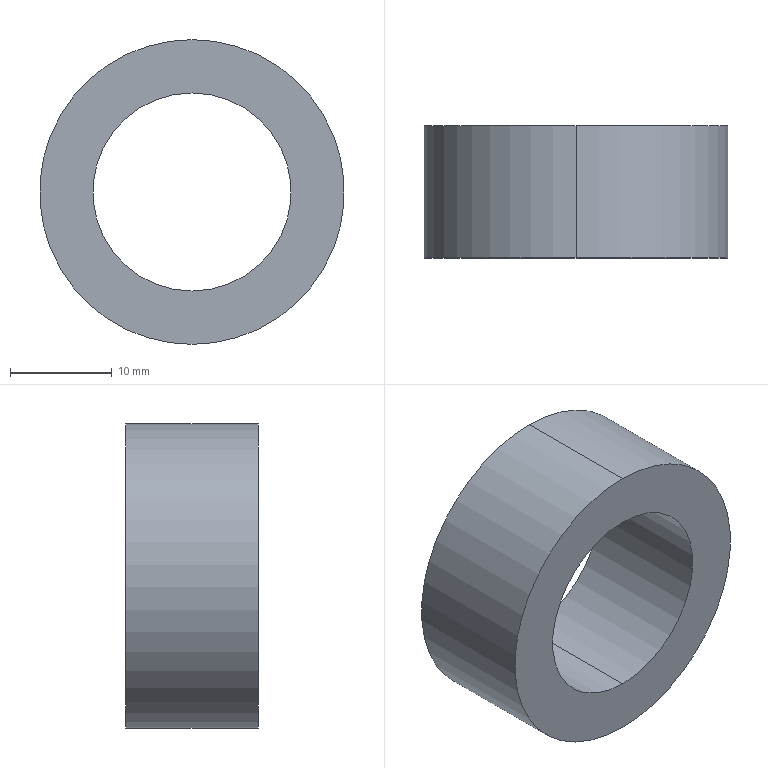Part | STEP file | Polyurethane washer | 1 solid | 6 faces | box 30 x 13 x 30 mm | volume 5307 mm3 | cylinder 4 | plane 2 | commonest cylinder face diameters 19.5 x2 30 x2
STEP:
#1=CARTESIAN_POINT('',(0.,0.,0.));
#2=DIRECTION('',(0.,0.,1.));
#3=DIRECTION('',(1.,0.,0.));
#4=AXIS2_PLACEMENT_3D('',#1,#2,#3);
#5=CARTESIAN_POINT('',(0.,13.,-9.75));
#6=VERTEX_POINT('',#5);
#7=CARTESIAN_POINT('',(0.,0.,-9.75));
#8=VERTEX_POINT('',#7);
#9=CARTESIAN_POINT('',(0.,13.,-9.75));
#10=DIRECTION('',(0.,-1.,0.));
#11=VECTOR('',#10,1.);
#12=LINE('',#9,#11);
#13=CARTESIAN_POINT('',(0.,13.,0.));
#14=DIRECTION('',(0.,-1.,0.));
#15=DIRECTION('',(0.,0.,-1.));
#16=AXIS2_PLACEMENT_3D('',#13,#14,#15);
#17=CYLINDRICAL_SURFACE('',#16,9.75);
#18=CARTESIAN_POINT('',(6.283,0.));
#19=DIRECTION('',(0.,1.));
#20=VECTOR('',#19,1.);
#21=LINE('',#18,#20);
#22=(GEOMETRIC_REPRESENTATION_CONTEXT(2)PARAMETRIC_REPRESENTATION_CONTEXT()REPRESENTATION_CONTEXT('',''));
#23=DEFINITIONAL_REPRESENTATION('',(#21),#22);
#24=PCURVE('',#17,#23);
#25=CARTESIAN_POINT('',(0.,13.,0.));
#26=DIRECTION('',(0.,-1.,0.));
#27=DIRECTION('',(0.,0.,-1.));
#28=AXIS2_PLACEMENT_3D('',#25,#26,#27);
#29=CYLINDRICAL_SURFACE('',#28,9.75);
#30=CARTESIAN_POINT('',(0.,0.));
#31=DIRECTION('',(0.,1.));
#32=VECTOR('',#31,1.);
#33=LINE('',#30,#32);
#34=(GEOMETRIC_REPRESENTATION_CONTEXT(2)PARAMETRIC_REPRESENTATION_CONTEXT()REPRESENTATION_CONTEXT('',''));
#35=DEFINITIONAL_REPRESENTATION('',(#33),#34);
#36=PCURVE('',#29,#35);
#37=SURFACE_CURVE('',#12,(#24,#36),.PCURVE_S1.);
#38=EDGE_CURVE('',#6,#8,#37,.T.);
#39=ORIENTED_EDGE('',*,*,#38,.T.);
#40=CARTESIAN_POINT('',(0.,0.,9.75));
#41=VERTEX_POINT('',#40);
#42=CARTESIAN_POINT('',(0.,0.,0.));
#43=DIRECTION('',(0.,1.,0.));
#44=DIRECTION('',(0.,0.,1.));
#45=AXIS2_PLACEMENT_3D('',#42,#43,#44);
#46=CIRCLE('',#45,9.75);
#47=CARTESIAN_POINT('',(9.425,13.));
#48=DIRECTION('',(-1.,0.));
#49=VECTOR('',#48,1.);
#50=LINE('',#47,#49);
#51=(GEOMETRIC_REPRESENTATION_CONTEXT(2)PARAMETRIC_REPRESENTATION_CONTEXT()REPRESENTATION_CONTEXT('',''));
#52=DEFINITIONAL_REPRESENTATION('',(#50),#51);
#53=PCURVE('',#17,#52);
#54=CARTESIAN_POINT('',(0.,0.,0.));
#55=DIRECTION('',(0.,1.,0.));
#56=DIRECTION('',(0.,0.,1.));
#57=AXIS2_PLACEMENT_3D('',#54,#55,#56);
#58=PLANE('',#57);
#59=CARTESIAN_POINT('',(0.,0.));
#60=DIRECTION('',(1.,0.));
#61=AXIS2_PLACEMENT_2D('',#59,#60);
#62=CIRCLE('',#61,9.75);
#63=(GEOMETRIC_REPRESENTATION_CONTEXT(2)PARAMETRIC_REPRESENTATION_CONTEXT()REPRESENTATION_CONTEXT('',''));
#64=DEFINITIONAL_REPRESENTATION('',(#62),#63);
#65=PCURVE('',#58,#64);
#66=SURFACE_CURVE('',#46,(#53,#65),.PCURVE_S1.);
#67=EDGE_CURVE('',#8,#41,#66,.T.);
#68=ORIENTED_EDGE('',*,*,#67,.T.);
#69=CARTESIAN_POINT('',(0.,13.,9.75));
#70=VERTEX_POINT('',#69);
#71=CARTESIAN_POINT('',(0.,13.,9.75));
#72=DIRECTION('',(0.,-1.,0.));
#73=VECTOR('',#72,1.);
#74=LINE('',#71,#73);
#75=CARTESIAN_POINT('',(3.142,0.));
#76=DIRECTION('',(0.,1.));
#77=VECTOR('',#76,1.);
#78=LINE('',#75,#77);
#79=(GEOMETRIC_REPRESENTATION_CONTEXT(2)PARAMETRIC_REPRESENTATION_CONTEXT()REPRESENTATION_CONTEXT('',''));
#80=DEFINITIONAL_REPRESENTATION('',(#78),#79);
#81=PCURVE('',#17,#80);
#82=CARTESIAN_POINT('',(3.142,0.));
#83=DIRECTION('',(0.,1.));
#84=VECTOR('',#83,1.);
#85=LINE('',#82,#84);
#86=(GEOMETRIC_REPRESENTATION_CONTEXT(2)PARAMETRIC_REPRESENTATION_CONTEXT()REPRESENTATION_CONTEXT('',''));
#87=DEFINITIONAL_REPRESENTATION('',(#85),#86);
#88=PCURVE('',#29,#87);
#89=SURFACE_CURVE('',#74,(#81,#88),.PCURVE_S1.);
#90=EDGE_CURVE('',#70,#41,#89,.T.);
#91=ORIENTED_EDGE('',*,*,#90,.F.);
#92=CARTESIAN_POINT('',(0.,13.,0.));
#93=DIRECTION('',(0.,1.,0.));
#94=DIRECTION('',(0.,0.,1.));
#95=AXIS2_PLACEMENT_3D('',#92,#93,#94);
#96=CIRCLE('',#95,9.75);
#97=CARTESIAN_POINT('',(9.425,0.));
#98=DIRECTION('',(-1.,0.));
#99=VECTOR('',#98,1.);
#100=LINE('',#97,#99);
#101=(GEOMETRIC_REPRESENTATION_CONTEXT(2)PARAMETRIC_REPRESENTATION_CONTEXT()REPRESENTATION_CONTEXT('',''));
#102=DEFINITIONAL_REPRESENTATION('',(#100),#101);
#103=PCURVE('',#17,#102);
#104=CARTESIAN_POINT('',(0.,13.,0.));
#105=DIRECTION('',(0.,1.,0.));
#106=DIRECTION('',(0.,0.,1.));
#107=AXIS2_PLACEMENT_3D('',#104,#105,#106);
#108=PLANE('',#107);
#109=CARTESIAN_POINT('',(0.,0.));
#110=DIRECTION('',(1.,0.));
#111=AXIS2_PLACEMENT_2D('',#109,#110);
#112=CIRCLE('',#111,9.75);
#113=(GEOMETRIC_REPRESENTATION_CONTEXT(2)PARAMETRIC_REPRESENTATION_CONTEXT()REPRESENTATION_CONTEXT('',''));
#114=DEFINITIONAL_REPRESENTATION('',(#112),#113);
#115=PCURVE('',#108,#114);
#116=SURFACE_CURVE('',#96,(#103,#115),.PCURVE_S1.);
#117=EDGE_CURVE('',#6,#70,#116,.T.);
#118=ORIENTED_EDGE('',*,*,#117,.F.);
#119=EDGE_LOOP('',(#39,#68,#91,#118));
#120=FACE_BOUND('',#119,.F.);
#121=ADVANCED_FACE('',(#120),#17,.F.);
#122=CARTESIAN_POINT('',(0.,13.,15.));
#123=VERTEX_POINT('',#122);
#124=CARTESIAN_POINT('',(0.,13.,-15.));
#125=VERTEX_POINT('',#124);
#126=CARTESIAN_POINT('',(0.,13.,0.));
#127=DIRECTION('',(0.,1.,0.));
#128=DIRECTION('',(0.,0.,1.));
#129=AXIS2_PLACEMENT_3D('',#126,#127,#128);
#130=CIRCLE('',#129,15.);
#131=CARTESIAN_POINT('',(0.,13.,0.));
#132=DIRECTION('',(0.,-1.,0.));
#133=DIRECTION('',(0.,0.,-1.));
#134=AXIS2_PLACEMENT_3D('',#131,#132,#133);
#135=CYLINDRICAL_SURFACE('',#134,15.);
#136=CARTESIAN_POINT('',(3.142,0.));
#137=DIRECTION('',(-1.,0.));
#138=VECTOR('',#137,1.);
#139=LINE('',#136,#138);
#140=(GEOMETRIC_REPRESENTATION_CONTEXT(2)PARAMETRIC_REPRESENTATION_CONTEXT()REPRESENTATION_CONTEXT('',''));
#141=DEFINITIONAL_REPRESENTATION('',(#139),#140);
#142=PCURVE('',#135,#141);
#143=CARTESIAN_POINT('',(0.,0.));
#144=DIRECTION('',(1.,0.));
#145=AXIS2_PLACEMENT_2D('',#143,#144);
#146=CIRCLE('',#145,15.);
#147=(GEOMETRIC_REPRESENTATION_CONTEXT(2)PARAMETRIC_REPRESENTATION_CONTEXT()REPRESENTATION_CONTEXT('',''));
#148=DEFINITIONAL_REPRESENTATION('',(#146),#147);
#149=PCURVE('',#108,#148);
#150=SURFACE_CURVE('',#130,(#142,#149),.PCURVE_S1.);
#151=EDGE_CURVE('',#123,#125,#150,.T.);
#152=ORIENTED_EDGE('',*,*,#151,.F.);
#153=CARTESIAN_POINT('',(0.,0.,15.));
#154=VERTEX_POINT('',#153);
#155=CARTESIAN_POINT('',(0.,13.,15.));
#156=DIRECTION('',(0.,-1.,0.));
#157=VECTOR('',#156,1.);
#158=LINE('',#155,#157);
#159=CARTESIAN_POINT('',(3.142,0.));
#160=DIRECTION('',(0.,1.));
#161=VECTOR('',#160,1.);
#162=LINE('',#159,#161);
#163=(GEOMETRIC_REPRESENTATION_CONTEXT(2)PARAMETRIC_REPRESENTATION_CONTEXT()REPRESENTATION_CONTEXT('',''));
#164=DEFINITIONAL_REPRESENTATION('',(#162),#163);
#165=PCURVE('',#135,#164);
#166=CARTESIAN_POINT('',(0.,13.,0.));
#167=DIRECTION('',(0.,-1.,0.));
#168=DIRECTION('',(0.,0.,-1.));
#169=AXIS2_PLACEMENT_3D('',#166,#167,#168);
#170=CYLINDRICAL_SURFACE('',#169,15.);
#171=CARTESIAN_POINT('',(3.142,0.));
#172=DIRECTION('',(0.,1.));
#173=VECTOR('',#172,1.);
#174=LINE('',#171,#173);
#175=(GEOMETRIC_REPRESENTATION_CONTEXT(2)PARAMETRIC_REPRESENTATION_CONTEXT()REPRESENTATION_CONTEXT('',''));
#176=DEFINITIONAL_REPRESENTATION('',(#174),#175);
#177=PCURVE('',#170,#176);
#178=SURFACE_CURVE('',#158,(#165,#177),.PCURVE_S1.);
#179=EDGE_CURVE('',#123,#154,#178,.T.);
#180=ORIENTED_EDGE('',*,*,#179,.T.);
#181=CARTESIAN_POINT('',(0.,0.,-15.));
#182=VERTEX_POINT('',#181);
#183=CARTESIAN_POINT('',(0.,0.,0.));
#184=DIRECTION('',(0.,1.,0.));
#185=DIRECTION('',(0.,0.,1.));
#186=AXIS2_PLACEMENT_3D('',#183,#184,#185);
#187=CIRCLE('',#186,15.);
#188=CARTESIAN_POINT('',(3.142,13.));
#189=DIRECTION('',(-1.,0.));
#190=VECTOR('',#189,1.);
#191=LINE('',#188,#190);
#192=(GEOMETRIC_REPRESENTATION_CONTEXT(2)PARAMETRIC_REPRESENTATION_CONTEXT()REPRESENTATION_CONTEXT('',''));
#193=DEFINITIONAL_REPRESENTATION('',(#191),#192);
#194=PCURVE('',#135,#193);
#195=CARTESIAN_POINT('',(0.,0.));
#196=DIRECTION('',(1.,0.));
#197=AXIS2_PLACEMENT_2D('',#195,#196);
#198=CIRCLE('',#197,15.);
#199=(GEOMETRIC_REPRESENTATION_CONTEXT(2)PARAMETRIC_REPRESENTATION_CONTEXT()REPRESENTATION_CONTEXT('',''));
#200=DEFINITIONAL_REPRESENTATION('',(#198),#199);
#201=PCURVE('',#58,#200);
#202=SURFACE_CURVE('',#187,(#194,#201),.PCURVE_S1.);
#203=EDGE_CURVE('',#154,#182,#202,.T.);
#204=ORIENTED_EDGE('',*,*,#203,.T.);
#205=CARTESIAN_POINT('',(0.,13.,-15.));
#206=DIRECTION('',(0.,-1.,0.));
#207=VECTOR('',#206,1.);
#208=LINE('',#205,#207);
#209=CARTESIAN_POINT('',(0.,0.));
#210=DIRECTION('',(0.,1.));
#211=VECTOR('',#210,1.);
#212=LINE('',#209,#211);
#213=(GEOMETRIC_REPRESENTATION_CONTEXT(2)PARAMETRIC_REPRESENTATION_CONTEXT()REPRESENTATION_CONTEXT('',''));
#214=DEFINITIONAL_REPRESENTATION('',(#212),#213);
#215=PCURVE('',#135,#214);
#216=CARTESIAN_POINT('',(6.283,0.));
#217=DIRECTION('',(0.,1.));
#218=VECTOR('',#217,1.);
#219=LINE('',#216,#218);
#220=(GEOMETRIC_REPRESENTATION_CONTEXT(2)PARAMETRIC_REPRESENTATION_CONTEXT()REPRESENTATION_CONTEXT('',''));
#221=DEFINITIONAL_REPRESENTATION('',(#219),#220);
#222=PCURVE('',#170,#221);
#223=SURFACE_CURVE('',#208,(#215,#222),.PCURVE_S1.);
#224=EDGE_CURVE('',#125,#182,#223,.T.);
#225=ORIENTED_EDGE('',*,*,#224,.F.);
#226=EDGE_LOOP('',(#152,#180,#204,#225));
#227=FACE_BOUND('',#226,.T.);
#228=ADVANCED_FACE('',(#227),#135,.T.);
#229=CARTESIAN_POINT('',(0.,13.,0.));
#230=DIRECTION('',(0.,1.,0.));
#231=DIRECTION('',(0.,0.,1.));
#232=AXIS2_PLACEMENT_3D('',#229,#230,#231);
#233=CIRCLE('',#232,15.);
#234=CARTESIAN_POINT('',(0.,0.));
#235=DIRECTION('',(1.,0.));
#236=AXIS2_PLACEMENT_2D('',#234,#235);
#237=CIRCLE('',#236,15.);
#238=(GEOMETRIC_REPRESENTATION_CONTEXT(2)PARAMETRIC_REPRESENTATION_CONTEXT()REPRESENTATION_CONTEXT('',''));
#239=DEFINITIONAL_REPRESENTATION('',(#237),#238);
#240=PCURVE('',#108,#239);
#241=CARTESIAN_POINT('',(9.425,0.));
#242=DIRECTION('',(-1.,0.));
#243=VECTOR('',#242,1.);
#244=LINE('',#241,#243);
#245=(GEOMETRIC_REPRESENTATION_CONTEXT(2)PARAMETRIC_REPRESENTATION_CONTEXT()REPRESENTATION_CONTEXT('',''));
#246=DEFINITIONAL_REPRESENTATION('',(#244),#245);
#247=PCURVE('',#170,#246);
#248=SURFACE_CURVE('',#233,(#240,#247),.PCURVE_S1.);
#249=EDGE_CURVE('',#125,#123,#248,.T.);
#250=ORIENTED_EDGE('',*,*,#249,.T.);
#251=ORIENTED_EDGE('',*,*,#151,.T.);
#252=EDGE_LOOP('',(#250,#251));
#253=FACE_BOUND('',#252,.T.);
#254=ORIENTED_EDGE('',*,*,#117,.F.);
#255=CARTESIAN_POINT('',(0.,13.,0.));
#256=DIRECTION('',(0.,1.,0.));
#257=DIRECTION('',(0.,0.,1.));
#258=AXIS2_PLACEMENT_3D('',#255,#256,#257);
#259=CIRCLE('',#258,9.75);
#260=CARTESIAN_POINT('',(0.,0.));
#261=DIRECTION('',(1.,0.));
#262=AXIS2_PLACEMENT_2D('',#260,#261);
#263=CIRCLE('',#262,9.75);
#264=(GEOMETRIC_REPRESENTATION_CONTEXT(2)PARAMETRIC_REPRESENTATION_CONTEXT()REPRESENTATION_CONTEXT('',''));
#265=DEFINITIONAL_REPRESENTATION('',(#263),#264);
#266=PCURVE('',#108,#265);
#267=CARTESIAN_POINT('',(3.142,0.));
#268=DIRECTION('',(-1.,0.));
#269=VECTOR('',#268,1.);
#270=LINE('',#267,#269);
#271=(GEOMETRIC_REPRESENTATION_CONTEXT(2)PARAMETRIC_REPRESENTATION_CONTEXT()REPRESENTATION_CONTEXT('',''));
#272=DEFINITIONAL_REPRESENTATION('',(#270),#271);
#273=PCURVE('',#29,#272);
#274=SURFACE_CURVE('',#259,(#266,#273),.PCURVE_S1.);
#275=EDGE_CURVE('',#70,#6,#274,.T.);
#276=ORIENTED_EDGE('',*,*,#275,.F.);
#277=EDGE_LOOP('',(#254,#276));
#278=FACE_BOUND('',#277,.T.);
#279=ADVANCED_FACE('',(#253,#278),#108,.T.);
#280=CARTESIAN_POINT('',(0.,0.,0.));
#281=DIRECTION('',(0.,1.,0.));
#282=DIRECTION('',(0.,0.,1.));
#283=AXIS2_PLACEMENT_3D('',#280,#281,#282);
#284=CIRCLE('',#283,15.);
#285=CARTESIAN_POINT('',(0.,0.));
#286=DIRECTION('',(1.,0.));
#287=AXIS2_PLACEMENT_2D('',#285,#286);
#288=CIRCLE('',#287,15.);
#289=(GEOMETRIC_REPRESENTATION_CONTEXT(2)PARAMETRIC_REPRESENTATION_CONTEXT()REPRESENTATION_CONTEXT('',''));
#290=DEFINITIONAL_REPRESENTATION('',(#288),#289);
#291=PCURVE('',#58,#290);
#292=CARTESIAN_POINT('',(9.425,13.));
#293=DIRECTION('',(-1.,0.));
#294=VECTOR('',#293,1.);
#295=LINE('',#292,#294);
#296=(GEOMETRIC_REPRESENTATION_CONTEXT(2)PARAMETRIC_REPRESENTATION_CONTEXT()REPRESENTATION_CONTEXT('',''));
#297=DEFINITIONAL_REPRESENTATION('',(#295),#296);
#298=PCURVE('',#170,#297);
#299=SURFACE_CURVE('',#284,(#291,#298),.PCURVE_S1.);
#300=EDGE_CURVE('',#182,#154,#299,.T.);
#301=ORIENTED_EDGE('',*,*,#300,.F.);
#302=ORIENTED_EDGE('',*,*,#203,.F.);
#303=EDGE_LOOP('',(#301,#302));
#304=FACE_BOUND('',#303,.T.);
#305=ORIENTED_EDGE('',*,*,#67,.T.);
#306=CARTESIAN_POINT('',(0.,0.,0.));
#307=DIRECTION('',(0.,1.,0.));
#308=DIRECTION('',(0.,0.,1.));
#309=AXIS2_PLACEMENT_3D('',#306,#307,#308);
#310=CIRCLE('',#309,9.75);
#311=CARTESIAN_POINT('',(0.,0.));
#312=DIRECTION('',(1.,0.));
#313=AXIS2_PLACEMENT_2D('',#311,#312);
#314=CIRCLE('',#313,9.75);
#315=(GEOMETRIC_REPRESENTATION_CONTEXT(2)PARAMETRIC_REPRESENTATION_CONTEXT()REPRESENTATION_CONTEXT('',''));
#316=DEFINITIONAL_REPRESENTATION('',(#314),#315);
#317=PCURVE('',#58,#316);
#318=CARTESIAN_POINT('',(3.142,13.));
#319=DIRECTION('',(-1.,0.));
#320=VECTOR('',#319,1.);
#321=LINE('',#318,#320);
#322=(GEOMETRIC_REPRESENTATION_CONTEXT(2)PARAMETRIC_REPRESENTATION_CONTEXT()REPRESENTATION_CONTEXT('',''));
#323=DEFINITIONAL_REPRESENTATION('',(#321),#322);
#324=PCURVE('',#29,#323);
#325=SURFACE_CURVE('',#310,(#317,#324),.PCURVE_S1.);
#326=EDGE_CURVE('',#41,#8,#325,.T.);
#327=ORIENTED_EDGE('',*,*,#326,.T.);
#328=EDGE_LOOP('',(#305,#327));
#329=FACE_BOUND('',#328,.T.);
#330=ADVANCED_FACE('',(#304,#329),#58,.F.);
#331=ORIENTED_EDGE('',*,*,#179,.F.);
#332=ORIENTED_EDGE('',*,*,#249,.F.);
#333=ORIENTED_EDGE('',*,*,#224,.T.);
#334=ORIENTED_EDGE('',*,*,#300,.T.);
#335=EDGE_LOOP('',(#331,#332,#333,#334));
#336=FACE_BOUND('',#335,.T.);
#337=ADVANCED_FACE('',(#336),#170,.T.);
#338=ORIENTED_EDGE('',*,*,#326,.T.);
#339=ORIENTED_EDGE('',*,*,#38,.F.);
#340=ORIENTED_EDGE('',*,*,#275,.F.);
#341=ORIENTED_EDGE('',*,*,#90,.T.);
#342=EDGE_LOOP('',(#338,#339,#340,#341));
#343=FACE_BOUND('',#342,.F.);
#344=ADVANCED_FACE('',(#343),#29,.F.);
#345=CLOSED_SHELL('',(#121,#228,#279,#330,#337,#344));
#346=MANIFOLD_SOLID_BREP('',#345);
#347=(LENGTH_UNIT()NAMED_UNIT(*)SI_UNIT(.MILLI.,.METRE.));
#348=UNCERTAINTY_MEASURE_WITH_UNIT(LENGTH_MEASURE(0.0000001),#347,'','');
#349=(NAMED_UNIT(*)PLANE_ANGLE_UNIT()SI_UNIT($,.RADIAN.));
#350=(NAMED_UNIT(*)SI_UNIT($,.STERADIAN.)SOLID_ANGLE_UNIT());
#351=(GEOMETRIC_REPRESENTATION_CONTEXT(3)GLOBAL_UNCERTAINTY_ASSIGNED_CONTEXT((#348))GLOBAL_UNIT_ASSIGNED_CONTEXT((#347,#349,#350))REPRESENTATION_CONTEXT('',''));
#352=ADVANCED_BREP_SHAPE_REPRESENTATION('',(#4,#346),#351);